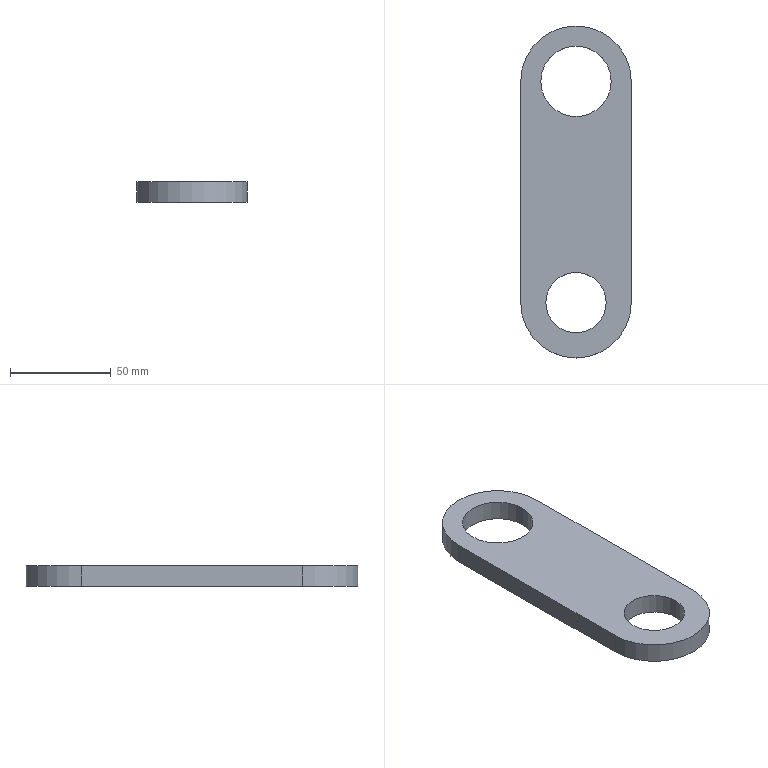Part | SolidWorks | features Extrusion 1 | 1 solid | 10 faces | box 55 x 165 x 10 mm | volume 67569 mm3 | cylinder 6 | plane 4 | commonest cylinder face diameters 30 x2 35 x2 55 x2
STEP:
#1=CARTESIAN_POINT('',(-17.5,110.,10.));
#2=VERTEX_POINT('',#1);
#3=CARTESIAN_POINT('',(17.5,110.,10.));
#4=VERTEX_POINT('',#3);
#5=CARTESIAN_POINT('',(0.,110.,10.));
#6=DIRECTION('',(0.,0.,1.));
#7=DIRECTION('',(1.,0.,0.));
#8=AXIS2_PLACEMENT_3D('',#5,#6,#7);
#9=CIRCLE('',#8,17.5);
#10=EDGE_CURVE('',#2,#4,#9,.T.);
#11=ORIENTED_EDGE('',*,*,#10,.T.);
#12=CARTESIAN_POINT('',(17.5,110.,0.));
#13=VERTEX_POINT('',#12);
#14=CARTESIAN_POINT('',(17.5,110.,10.));
#15=DIRECTION('',(0.,0.,-1.));
#16=VECTOR('',#15,1000.);
#17=LINE('',#14,#16);
#18=EDGE_CURVE('',#4,#13,#17,.T.);
#19=ORIENTED_EDGE('',*,*,#18,.T.);
#20=CARTESIAN_POINT('',(-17.5,110.,0.));
#21=VERTEX_POINT('',#20);
#22=CARTESIAN_POINT('',(0.,110.,0.));
#23=DIRECTION('',(0.,0.,1.));
#24=DIRECTION('',(1.,0.,0.));
#25=AXIS2_PLACEMENT_3D('',#22,#23,#24);
#26=CIRCLE('',#25,17.5);
#27=EDGE_CURVE('',#21,#13,#26,.T.);
#28=ORIENTED_EDGE('',*,*,#27,.F.);
#29=CARTESIAN_POINT('',(-17.5,110.,10.));
#30=DIRECTION('',(0.,0.,-1.));
#31=VECTOR('',#30,1000.);
#32=LINE('',#29,#31);
#33=EDGE_CURVE('',#2,#21,#32,.T.);
#34=ORIENTED_EDGE('',*,*,#33,.F.);
#35=EDGE_LOOP('',(#11,#19,#28,#34));
#36=FACE_OUTER_BOUND('',#35,.T.);
#37=CARTESIAN_POINT('',(0.,110.,10.));
#38=DIRECTION('',(0.,0.,-1.));
#39=DIRECTION('',(-1.,0.,0.));
#40=AXIS2_PLACEMENT_3D('',#37,#38,#39);
#41=CYLINDRICAL_SURFACE('',#40,17.5);
#42=ADVANCED_FACE('',(#36),#41,.F.);
#43=CARTESIAN_POINT('',(-15.,0.,10.));
#44=VERTEX_POINT('',#43);
#45=CARTESIAN_POINT('',(15.,0.,10.));
#46=VERTEX_POINT('',#45);
#47=CARTESIAN_POINT('',(0.,0.,10.));
#48=DIRECTION('',(0.,0.,1.));
#49=DIRECTION('',(1.,0.,0.));
#50=AXIS2_PLACEMENT_3D('',#47,#48,#49);
#51=CIRCLE('',#50,15.);
#52=EDGE_CURVE('',#44,#46,#51,.T.);
#53=ORIENTED_EDGE('',*,*,#52,.T.);
#54=CARTESIAN_POINT('',(15.,0.,0.));
#55=VERTEX_POINT('',#54);
#56=CARTESIAN_POINT('',(15.,0.,10.));
#57=DIRECTION('',(0.,0.,-1.));
#58=VECTOR('',#57,1000.);
#59=LINE('',#56,#58);
#60=EDGE_CURVE('',#46,#55,#59,.T.);
#61=ORIENTED_EDGE('',*,*,#60,.T.);
#62=CARTESIAN_POINT('',(-15.,0.,0.));
#63=VERTEX_POINT('',#62);
#64=CARTESIAN_POINT('',(0.,0.,0.));
#65=DIRECTION('',(0.,0.,1.));
#66=DIRECTION('',(1.,0.,0.));
#67=AXIS2_PLACEMENT_3D('',#64,#65,#66);
#68=CIRCLE('',#67,15.);
#69=EDGE_CURVE('',#63,#55,#68,.T.);
#70=ORIENTED_EDGE('',*,*,#69,.F.);
#71=CARTESIAN_POINT('',(-15.,0.,10.));
#72=DIRECTION('',(0.,0.,-1.));
#73=VECTOR('',#72,1000.);
#74=LINE('',#71,#73);
#75=EDGE_CURVE('',#44,#63,#74,.T.);
#76=ORIENTED_EDGE('',*,*,#75,.F.);
#77=EDGE_LOOP('',(#53,#61,#70,#76));
#78=FACE_OUTER_BOUND('',#77,.T.);
#79=CARTESIAN_POINT('',(0.,0.,10.));
#80=DIRECTION('',(0.,0.,-1.));
#81=DIRECTION('',(-1.,0.,0.));
#82=AXIS2_PLACEMENT_3D('',#79,#80,#81);
#83=CYLINDRICAL_SURFACE('',#82,15.);
#84=ADVANCED_FACE('',(#78),#83,.F.);
#85=ORIENTED_EDGE('',*,*,#52,.F.);
#86=CARTESIAN_POINT('',(0.,0.,10.));
#87=DIRECTION('',(0.,0.,1.));
#88=DIRECTION('',(1.,0.,0.));
#89=AXIS2_PLACEMENT_3D('',#86,#87,#88);
#90=CIRCLE('',#89,15.);
#91=EDGE_CURVE('',#46,#44,#90,.T.);
#92=ORIENTED_EDGE('',*,*,#91,.F.);
#93=EDGE_LOOP('',(#85,#92));
#94=FACE_BOUND('',#93,.T.);
#95=CARTESIAN_POINT('',(27.5,110.,10.));
#96=VERTEX_POINT('',#95);
#97=CARTESIAN_POINT('',(-27.5,110.,10.));
#98=VERTEX_POINT('',#97);
#99=CARTESIAN_POINT('',(0.,110.,10.));
#100=DIRECTION('',(0.,0.,1.));
#101=DIRECTION('',(1.,0.,0.));
#102=AXIS2_PLACEMENT_3D('',#99,#100,#101);
#103=CIRCLE('',#102,27.5);
#104=EDGE_CURVE('',#96,#98,#103,.T.);
#105=ORIENTED_EDGE('',*,*,#104,.T.);
#106=CARTESIAN_POINT('',(-27.5,0.,10.));
#107=VERTEX_POINT('',#106);
#108=CARTESIAN_POINT('',(-27.5,110.,10.));
#109=DIRECTION('',(0.,-1.,0.));
#110=VECTOR('',#109,1000.);
#111=LINE('',#108,#110);
#112=EDGE_CURVE('',#98,#107,#111,.T.);
#113=ORIENTED_EDGE('',*,*,#112,.T.);
#114=CARTESIAN_POINT('',(27.5,0.,10.));
#115=VERTEX_POINT('',#114);
#116=CARTESIAN_POINT('',(0.,0.,10.));
#117=DIRECTION('',(0.,0.,1.));
#118=DIRECTION('',(1.,0.,0.));
#119=AXIS2_PLACEMENT_3D('',#116,#117,#118);
#120=CIRCLE('',#119,27.5);
#121=EDGE_CURVE('',#107,#115,#120,.T.);
#122=ORIENTED_EDGE('',*,*,#121,.T.);
#123=CARTESIAN_POINT('',(27.5,110.,10.));
#124=DIRECTION('',(0.,1.,0.));
#125=VECTOR('',#124,1000.);
#126=LINE('',#123,#125);
#127=EDGE_CURVE('',#115,#96,#126,.T.);
#128=ORIENTED_EDGE('',*,*,#127,.T.);
#129=EDGE_LOOP('',(#105,#113,#122,#128));
#130=FACE_OUTER_BOUND('',#129,.T.);
#131=ORIENTED_EDGE('',*,*,#10,.F.);
#132=CARTESIAN_POINT('',(0.,110.,10.));
#133=DIRECTION('',(0.,0.,1.));
#134=DIRECTION('',(1.,0.,0.));
#135=AXIS2_PLACEMENT_3D('',#132,#133,#134);
#136=CIRCLE('',#135,17.5);
#137=EDGE_CURVE('',#4,#2,#136,.T.);
#138=ORIENTED_EDGE('',*,*,#137,.F.);
#139=EDGE_LOOP('',(#131,#138));
#140=FACE_BOUND('',#139,.T.);
#141=CARTESIAN_POINT('',(0.,110.,10.));
#142=DIRECTION('',(0.,0.,1.));
#143=DIRECTION('',(1.,0.,0.));
#144=AXIS2_PLACEMENT_3D('',#141,#142,#143);
#145=PLANE('',#144);
#146=ADVANCED_FACE('',(#94,#130,#140),#145,.T.);
#147=CARTESIAN_POINT('',(27.5,110.,0.));
#148=VERTEX_POINT('',#147);
#149=CARTESIAN_POINT('',(-27.5,110.,0.));
#150=VERTEX_POINT('',#149);
#151=CARTESIAN_POINT('',(0.,110.,0.));
#152=DIRECTION('',(0.,0.,1.));
#153=DIRECTION('',(1.,0.,0.));
#154=AXIS2_PLACEMENT_3D('',#151,#152,#153);
#155=CIRCLE('',#154,27.5);
#156=EDGE_CURVE('',#148,#150,#155,.T.);
#157=ORIENTED_EDGE('',*,*,#156,.F.);
#158=CARTESIAN_POINT('',(27.5,0.,0.));
#159=VERTEX_POINT('',#158);
#160=CARTESIAN_POINT('',(27.5,110.,0.));
#161=DIRECTION('',(0.,1.,0.));
#162=VECTOR('',#161,1000.);
#163=LINE('',#160,#162);
#164=EDGE_CURVE('',#159,#148,#163,.T.);
#165=ORIENTED_EDGE('',*,*,#164,.F.);
#166=CARTESIAN_POINT('',(-27.5,0.,0.));
#167=VERTEX_POINT('',#166);
#168=CARTESIAN_POINT('',(0.,0.,0.));
#169=DIRECTION('',(0.,0.,1.));
#170=DIRECTION('',(1.,0.,0.));
#171=AXIS2_PLACEMENT_3D('',#168,#169,#170);
#172=CIRCLE('',#171,27.5);
#173=EDGE_CURVE('',#167,#159,#172,.T.);
#174=ORIENTED_EDGE('',*,*,#173,.F.);
#175=CARTESIAN_POINT('',(-27.5,110.,0.));
#176=DIRECTION('',(0.,-1.,0.));
#177=VECTOR('',#176,1000.);
#178=LINE('',#175,#177);
#179=EDGE_CURVE('',#150,#167,#178,.T.);
#180=ORIENTED_EDGE('',*,*,#179,.F.);
#181=EDGE_LOOP('',(#157,#165,#174,#180));
#182=FACE_OUTER_BOUND('',#181,.T.);
#183=ORIENTED_EDGE('',*,*,#69,.T.);
#184=CARTESIAN_POINT('',(0.,0.,0.));
#185=DIRECTION('',(0.,0.,1.));
#186=DIRECTION('',(1.,0.,0.));
#187=AXIS2_PLACEMENT_3D('',#184,#185,#186);
#188=CIRCLE('',#187,15.);
#189=EDGE_CURVE('',#55,#63,#188,.T.);
#190=ORIENTED_EDGE('',*,*,#189,.T.);
#191=EDGE_LOOP('',(#183,#190));
#192=FACE_BOUND('',#191,.T.);
#193=ORIENTED_EDGE('',*,*,#27,.T.);
#194=CARTESIAN_POINT('',(0.,110.,0.));
#195=DIRECTION('',(0.,0.,1.));
#196=DIRECTION('',(1.,0.,0.));
#197=AXIS2_PLACEMENT_3D('',#194,#195,#196);
#198=CIRCLE('',#197,17.5);
#199=EDGE_CURVE('',#13,#21,#198,.T.);
#200=ORIENTED_EDGE('',*,*,#199,.T.);
#201=EDGE_LOOP('',(#193,#200));
#202=FACE_BOUND('',#201,.T.);
#203=CARTESIAN_POINT('',(0.,110.,0.));
#204=DIRECTION('',(0.,0.,1.));
#205=DIRECTION('',(1.,0.,0.));
#206=AXIS2_PLACEMENT_3D('',#203,#204,#205);
#207=PLANE('',#206);
#208=ADVANCED_FACE('',(#182,#192,#202),#207,.F.);
#209=ORIENTED_EDGE('',*,*,#156,.T.);
#210=CARTESIAN_POINT('',(-27.5,110.,10.));
#211=DIRECTION('',(0.,0.,-1.));
#212=VECTOR('',#211,1000.);
#213=LINE('',#210,#212);
#214=EDGE_CURVE('',#98,#150,#213,.T.);
#215=ORIENTED_EDGE('',*,*,#214,.F.);
#216=ORIENTED_EDGE('',*,*,#104,.F.);
#217=CARTESIAN_POINT('',(27.5,110.,10.));
#218=DIRECTION('',(0.,0.,-1.));
#219=VECTOR('',#218,1000.);
#220=LINE('',#217,#219);
#221=EDGE_CURVE('',#96,#148,#220,.T.);
#222=ORIENTED_EDGE('',*,*,#221,.T.);
#223=EDGE_LOOP('',(#209,#215,#216,#222));
#224=FACE_OUTER_BOUND('',#223,.T.);
#225=CARTESIAN_POINT('',(0.,110.,10.));
#226=DIRECTION('',(0.,0.,-1.));
#227=DIRECTION('',(-1.,0.,0.));
#228=AXIS2_PLACEMENT_3D('',#225,#226,#227);
#229=CYLINDRICAL_SURFACE('',#228,27.5);
#230=ADVANCED_FACE('',(#224),#229,.T.);
#231=ORIENTED_EDGE('',*,*,#179,.T.);
#232=CARTESIAN_POINT('',(-27.5,0.,10.));
#233=DIRECTION('',(0.,0.,-1.));
#234=VECTOR('',#233,1000.);
#235=LINE('',#232,#234);
#236=EDGE_CURVE('',#107,#167,#235,.T.);
#237=ORIENTED_EDGE('',*,*,#236,.F.);
#238=ORIENTED_EDGE('',*,*,#112,.F.);
#239=ORIENTED_EDGE('',*,*,#214,.T.);
#240=EDGE_LOOP('',(#231,#237,#238,#239));
#241=FACE_OUTER_BOUND('',#240,.T.);
#242=CARTESIAN_POINT('',(-27.5,110.,10.));
#243=DIRECTION('',(1.,0.,0.));
#244=DIRECTION('',(0.,1.,0.));
#245=AXIS2_PLACEMENT_3D('',#242,#243,#244);
#246=PLANE('',#245);
#247=ADVANCED_FACE('',(#241),#246,.F.);
#248=ORIENTED_EDGE('',*,*,#173,.T.);
#249=CARTESIAN_POINT('',(27.5,0.,10.));
#250=DIRECTION('',(0.,0.,-1.));
#251=VECTOR('',#250,1000.);
#252=LINE('',#249,#251);
#253=EDGE_CURVE('',#115,#159,#252,.T.);
#254=ORIENTED_EDGE('',*,*,#253,.F.);
#255=ORIENTED_EDGE('',*,*,#121,.F.);
#256=ORIENTED_EDGE('',*,*,#236,.T.);
#257=EDGE_LOOP('',(#248,#254,#255,#256));
#258=FACE_OUTER_BOUND('',#257,.T.);
#259=CARTESIAN_POINT('',(0.,0.,10.));
#260=DIRECTION('',(0.,0.,-1.));
#261=DIRECTION('',(-1.,0.,0.));
#262=AXIS2_PLACEMENT_3D('',#259,#260,#261);
#263=CYLINDRICAL_SURFACE('',#262,27.5);
#264=ADVANCED_FACE('',(#258),#263,.T.);
#265=ORIENTED_EDGE('',*,*,#164,.T.);
#266=ORIENTED_EDGE('',*,*,#221,.F.);
#267=ORIENTED_EDGE('',*,*,#127,.F.);
#268=ORIENTED_EDGE('',*,*,#253,.T.);
#269=EDGE_LOOP('',(#265,#266,#267,#268));
#270=FACE_OUTER_BOUND('',#269,.T.);
#271=CARTESIAN_POINT('',(27.5,110.,10.));
#272=DIRECTION('',(-1.,0.,0.));
#273=DIRECTION('',(0.,-1.,0.));
#274=AXIS2_PLACEMENT_3D('',#271,#272,#273);
#275=PLANE('',#274);
#276=ADVANCED_FACE('',(#270),#275,.F.);
#277=ORIENTED_EDGE('',*,*,#60,.F.);
#278=ORIENTED_EDGE('',*,*,#91,.T.);
#279=ORIENTED_EDGE('',*,*,#75,.T.);
#280=ORIENTED_EDGE('',*,*,#189,.F.);
#281=EDGE_LOOP('',(#277,#278,#279,#280));
#282=FACE_OUTER_BOUND('',#281,.T.);
#283=CARTESIAN_POINT('',(0.,0.,10.));
#284=DIRECTION('',(0.,0.,-1.));
#285=DIRECTION('',(-1.,0.,0.));
#286=AXIS2_PLACEMENT_3D('',#283,#284,#285);
#287=CYLINDRICAL_SURFACE('',#286,15.);
#288=ADVANCED_FACE('',(#282),#287,.F.);
#289=ORIENTED_EDGE('',*,*,#18,.F.);
#290=ORIENTED_EDGE('',*,*,#137,.T.);
#291=ORIENTED_EDGE('',*,*,#33,.T.);
#292=ORIENTED_EDGE('',*,*,#199,.F.);
#293=EDGE_LOOP('',(#289,#290,#291,#292));
#294=FACE_OUTER_BOUND('',#293,.T.);
#295=CARTESIAN_POINT('',(0.,110.,10.));
#296=DIRECTION('',(0.,0.,-1.));
#297=DIRECTION('',(-1.,0.,0.));
#298=AXIS2_PLACEMENT_3D('',#295,#296,#297);
#299=CYLINDRICAL_SURFACE('',#298,17.5);
#300=ADVANCED_FACE('',(#294),#299,.F.);
#301=CLOSED_SHELL('',(#42,#84,#146,#208,#230,#247,#264,#276,#288,#300));
#302=MANIFOLD_SOLID_BREP('',#301);
#303=CARTESIAN_POINT('',(0.,0.,0.));
#304=DIRECTION('',(0.,0.,1.));
#305=DIRECTION('',(1.,0.,0.));
#306=AXIS2_PLACEMENT_3D('',#303,#304,#305);
#307=(LENGTH_UNIT()NAMED_UNIT(*)SI_UNIT(.MILLI.,.METRE.));
#308=UNCERTAINTY_MEASURE_WITH_UNIT(LENGTH_MEASURE(0.00001),#307,'','');
#309=(NAMED_UNIT(*)PLANE_ANGLE_UNIT()SI_UNIT($,.RADIAN.));
#310=(NAMED_UNIT(*)SI_UNIT($,.STERADIAN.)SOLID_ANGLE_UNIT());
#311=(GEOMETRIC_REPRESENTATION_CONTEXT(3)GLOBAL_UNCERTAINTY_ASSIGNED_CONTEXT((#308))GLOBAL_UNIT_ASSIGNED_CONTEXT((#307,#309,#310))REPRESENTATION_CONTEXT('',''));
#312=ADVANCED_BREP_SHAPE_REPRESENTATION('',(#302,#306),#311);